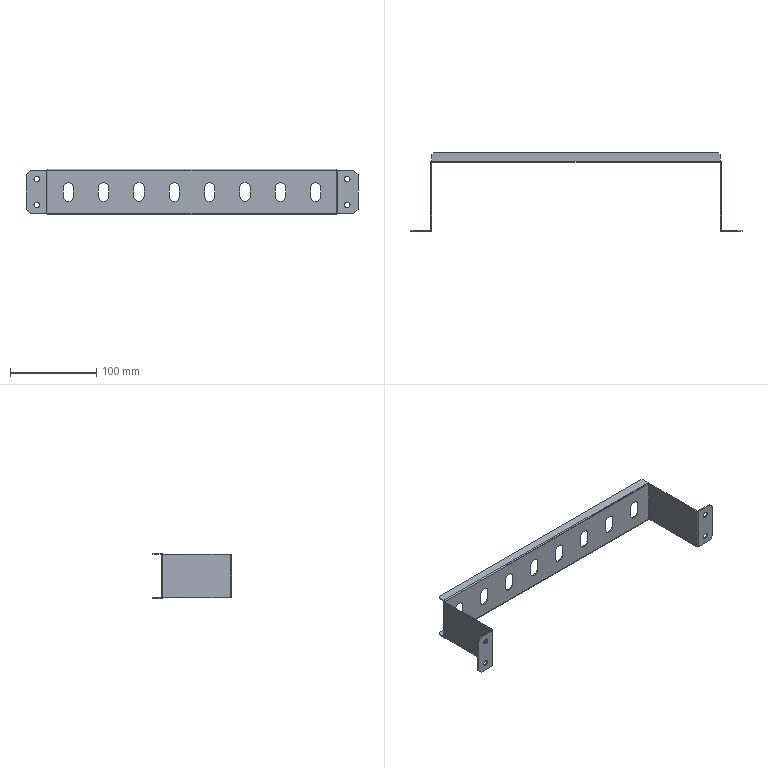Part | SolidWorks | features CornerTrim 2, ICE 2, EdgeFlange 1, FlatPattern 1, LPattern 1, MirrorPattern 1, SMBaseFlange 1, SheetMetal 1 | 1 solid | 110 faces | box 385 x 91.2 x 52.6 mm | volume 39000 mm3 | plane 66 | cylinder 44 | commonest cylinder face diameters 12 x24 6.5 x8 0.2 x6 2.6 x6